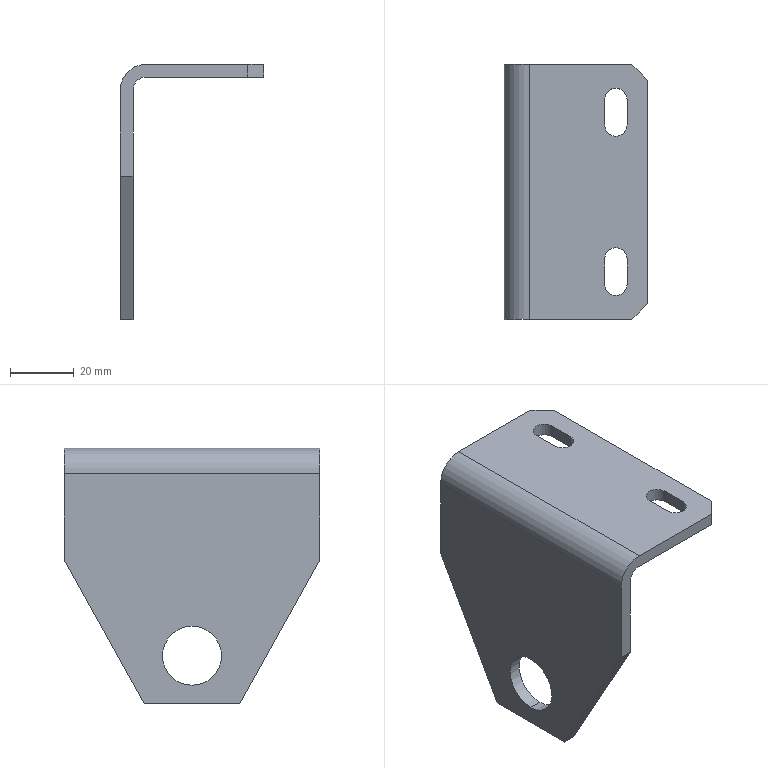Part | SolidWorks | features ICE 3, Chamfer 2, Fillet 2, Extrusion 1, HoleWzd 1 | 1 solid | 24 faces | box 45 x 80 x 80 mm | volume 31465 mm3 | plane 16 | cylinder 8 | commonest cylinder face diameters 7 x4 18.5 x2 8 x1 16 x1
STEP:
#1=CARTESIAN_POINT('',(-4.,40.,24.25));
#2=VERTEX_POINT('',#1);
#3=CARTESIAN_POINT('',(-4.,40.,5.75));
#4=VERTEX_POINT('',#3);
#5=CARTESIAN_POINT('',(-4.,40.,15.));
#6=DIRECTION('',(1.,0.,0.));
#7=DIRECTION('',(0.,0.,-1.));
#8=AXIS2_PLACEMENT_3D('',#5,#6,#7);
#9=CIRCLE('',#8,9.25);
#10=EDGE_CURVE('',#2,#4,#9,.T.);
#11=ORIENTED_EDGE('',*,*,#10,.F.);
#12=CARTESIAN_POINT('',(0.,40.,24.25));
#13=VERTEX_POINT('',#12);
#14=CARTESIAN_POINT('',(0.,40.,24.25));
#15=DIRECTION('',(1.,0.,0.));
#16=VECTOR('',#15,1000.);
#17=LINE('',#14,#16);
#18=EDGE_CURVE('',#2,#13,#17,.T.);
#19=ORIENTED_EDGE('',*,*,#18,.T.);
#20=CARTESIAN_POINT('',(0.,40.,5.75));
#21=VERTEX_POINT('',#20);
#22=CARTESIAN_POINT('',(0.,40.,15.));
#23=DIRECTION('',(1.,0.,0.));
#24=DIRECTION('',(0.,0.,-1.));
#25=AXIS2_PLACEMENT_3D('',#22,#23,#24);
#26=CIRCLE('',#25,9.25);
#27=EDGE_CURVE('',#13,#21,#26,.T.);
#28=ORIENTED_EDGE('',*,*,#27,.T.);
#29=CARTESIAN_POINT('',(0.,40.,5.75));
#30=DIRECTION('',(1.,0.,0.));
#31=VECTOR('',#30,1000.);
#32=LINE('',#29,#31);
#33=EDGE_CURVE('',#4,#21,#32,.T.);
#34=ORIENTED_EDGE('',*,*,#33,.F.);
#35=EDGE_LOOP('',(#11,#19,#28,#34));
#36=FACE_OUTER_BOUND('',#35,.T.);
#37=CARTESIAN_POINT('',(0.,40.,15.));
#38=DIRECTION('',(1.,0.,0.));
#39=DIRECTION('',(0.,0.,-1.));
#40=AXIS2_PLACEMENT_3D('',#37,#38,#39);
#41=CYLINDRICAL_SURFACE('',#40,9.25);
#42=ADVANCED_FACE('',(#36),#41,.F.);
#43=CARTESIAN_POINT('',(-4.,0.,72.));
#44=VERTEX_POINT('',#43);
#45=CARTESIAN_POINT('',(-4.,0.,45.));
#46=VERTEX_POINT('',#45);
#47=CARTESIAN_POINT('',(-4.,0.,80.));
#48=DIRECTION('',(0.,0.,-1.));
#49=VECTOR('',#48,1000.);
#50=LINE('',#47,#49);
#51=EDGE_CURVE('',#44,#46,#50,.T.);
#52=ORIENTED_EDGE('',*,*,#51,.F.);
#53=CARTESIAN_POINT('',(-4.,80.,72.));
#54=VERTEX_POINT('',#53);
#55=CARTESIAN_POINT('',(-4.,0.,72.));
#56=DIRECTION('',(0.,1.,0.));
#57=VECTOR('',#56,1000.);
#58=LINE('',#55,#57);
#59=EDGE_CURVE('',#44,#54,#58,.T.);
#60=ORIENTED_EDGE('',*,*,#59,.T.);
#61=CARTESIAN_POINT('',(-4.,80.,45.));
#62=VERTEX_POINT('',#61);
#63=CARTESIAN_POINT('',(-4.,80.,45.));
#64=DIRECTION('',(0.,0.,1.));
#65=VECTOR('',#64,1000.);
#66=LINE('',#63,#65);
#67=EDGE_CURVE('',#62,#54,#66,.T.);
#68=ORIENTED_EDGE('',*,*,#67,.F.);
#69=CARTESIAN_POINT('',(-4.,55.,0.));
#70=VERTEX_POINT('',#69);
#71=CARTESIAN_POINT('',(-4.,40.,-27.));
#72=DIRECTION('',(0.,0.4856,0.8742));
#73=VECTOR('',#72,1000.);
#74=LINE('',#71,#73);
#75=EDGE_CURVE('',#70,#62,#74,.T.);
#76=ORIENTED_EDGE('',*,*,#75,.F.);
#77=CARTESIAN_POINT('',(-4.,25.,0.));
#78=VERTEX_POINT('',#77);
#79=CARTESIAN_POINT('',(-4.,0.,0.));
#80=DIRECTION('',(0.,-1.,0.));
#81=VECTOR('',#80,1000.);
#82=LINE('',#79,#81);
#83=EDGE_CURVE('',#70,#78,#82,.T.);
#84=ORIENTED_EDGE('',*,*,#83,.T.);
#85=CARTESIAN_POINT('',(-4.,0.,45.));
#86=DIRECTION('',(0.,0.4856,-0.8742));
#87=VECTOR('',#86,1000.);
#88=LINE('',#85,#87);
#89=EDGE_CURVE('',#46,#78,#88,.T.);
#90=ORIENTED_EDGE('',*,*,#89,.F.);
#91=EDGE_LOOP('',(#52,#60,#68,#76,#84,#90));
#92=FACE_OUTER_BOUND('',#91,.T.);
#93=CARTESIAN_POINT('',(-4.,40.,15.));
#94=DIRECTION('',(1.,0.,0.));
#95=DIRECTION('',(0.,0.,-1.));
#96=AXIS2_PLACEMENT_3D('',#93,#94,#95);
#97=CIRCLE('',#96,9.25);
#98=EDGE_CURVE('',#4,#2,#97,.T.);
#99=ORIENTED_EDGE('',*,*,#98,.T.);
#100=ORIENTED_EDGE('',*,*,#10,.T.);
#101=EDGE_LOOP('',(#99,#100));
#102=FACE_BOUND('',#101,.T.);
#103=CARTESIAN_POINT('',(-4.,0.,0.));
#104=DIRECTION('',(-1.,0.,0.));
#105=DIRECTION('',(0.,0.,1.));
#106=AXIS2_PLACEMENT_3D('',#103,#104,#105);
#107=PLANE('',#106);
#108=ADVANCED_FACE('',(#92,#102),#107,.T.);
#109=CARTESIAN_POINT('',(0.,40.,15.));
#110=DIRECTION('',(1.,0.,0.));
#111=DIRECTION('',(0.,0.,-1.));
#112=AXIS2_PLACEMENT_3D('',#109,#110,#111);
#113=CIRCLE('',#112,9.25);
#114=EDGE_CURVE('',#21,#13,#113,.T.);
#115=ORIENTED_EDGE('',*,*,#114,.F.);
#116=ORIENTED_EDGE('',*,*,#27,.F.);
#117=EDGE_LOOP('',(#115,#116));
#118=FACE_BOUND('',#117,.T.);
#119=CARTESIAN_POINT('',(0.,80.,45.));
#120=VERTEX_POINT('',#119);
#121=CARTESIAN_POINT('',(0.,80.,72.));
#122=VERTEX_POINT('',#121);
#123=CARTESIAN_POINT('',(0.,80.,45.));
#124=DIRECTION('',(0.,0.,1.));
#125=VECTOR('',#124,1000.);
#126=LINE('',#123,#125);
#127=EDGE_CURVE('',#120,#122,#126,.T.);
#128=ORIENTED_EDGE('',*,*,#127,.T.);
#129=CARTESIAN_POINT('',(0.,0.,72.));
#130=VERTEX_POINT('',#129);
#131=CARTESIAN_POINT('',(0.,0.,72.));
#132=DIRECTION('',(0.,-1.,0.));
#133=VECTOR('',#132,1000.);
#134=LINE('',#131,#133);
#135=EDGE_CURVE('',#122,#130,#134,.T.);
#136=ORIENTED_EDGE('',*,*,#135,.T.);
#137=CARTESIAN_POINT('',(0.,0.,45.));
#138=VERTEX_POINT('',#137);
#139=CARTESIAN_POINT('',(0.,0.,80.));
#140=DIRECTION('',(0.,0.,-1.));
#141=VECTOR('',#140,1000.);
#142=LINE('',#139,#141);
#143=EDGE_CURVE('',#130,#138,#142,.T.);
#144=ORIENTED_EDGE('',*,*,#143,.T.);
#145=CARTESIAN_POINT('',(0.,25.,0.));
#146=VERTEX_POINT('',#145);
#147=CARTESIAN_POINT('',(0.,0.,45.));
#148=DIRECTION('',(0.,0.4856,-0.8742));
#149=VECTOR('',#148,1000.);
#150=LINE('',#147,#149);
#151=EDGE_CURVE('',#138,#146,#150,.T.);
#152=ORIENTED_EDGE('',*,*,#151,.T.);
#153=CARTESIAN_POINT('',(0.,55.,0.));
#154=VERTEX_POINT('',#153);
#155=CARTESIAN_POINT('',(0.,25.,0.));
#156=DIRECTION('',(0.,1.,0.));
#157=VECTOR('',#156,1000.);
#158=LINE('',#155,#157);
#159=EDGE_CURVE('',#146,#154,#158,.T.);
#160=ORIENTED_EDGE('',*,*,#159,.T.);
#161=CARTESIAN_POINT('',(0.,40.,-27.));
#162=DIRECTION('',(0.,0.4856,0.8742));
#163=VECTOR('',#162,1000.);
#164=LINE('',#161,#163);
#165=EDGE_CURVE('',#154,#120,#164,.T.);
#166=ORIENTED_EDGE('',*,*,#165,.T.);
#167=EDGE_LOOP('',(#128,#136,#144,#152,#160,#166));
#168=FACE_OUTER_BOUND('',#167,.T.);
#169=CARTESIAN_POINT('',(0.,0.,0.));
#170=DIRECTION('',(-1.,0.,0.));
#171=DIRECTION('',(0.,0.,1.));
#172=AXIS2_PLACEMENT_3D('',#169,#170,#171);
#173=PLANE('',#172);
#174=ADVANCED_FACE('',(#118,#168),#173,.F.);
#175=CARTESIAN_POINT('',(4.,0.,80.));
#176=VERTEX_POINT('',#175);
#177=CARTESIAN_POINT('',(36.,0.,80.));
#178=VERTEX_POINT('',#177);
#179=CARTESIAN_POINT('',(-4.,0.,80.));
#180=DIRECTION('',(1.,0.,0.));
#181=VECTOR('',#180,1000.);
#182=LINE('',#179,#181);
#183=EDGE_CURVE('',#176,#178,#182,.T.);
#184=ORIENTED_EDGE('',*,*,#183,.F.);
#185=CARTESIAN_POINT('',(4.,0.,72.));
#186=DIRECTION('',(0.,-1.,0.));
#187=DIRECTION('',(0.,0.,-1.));
#188=AXIS2_PLACEMENT_3D('',#185,#186,#187);
#189=CIRCLE('',#188,8.);
#190=EDGE_CURVE('',#176,#44,#189,.T.);
#191=ORIENTED_EDGE('',*,*,#190,.T.);
#192=ORIENTED_EDGE('',*,*,#51,.T.);
#193=CARTESIAN_POINT('',(-4.,0.,45.));
#194=DIRECTION('',(1.,0.,0.));
#195=VECTOR('',#194,1000.);
#196=LINE('',#193,#195);
#197=EDGE_CURVE('',#46,#138,#196,.T.);
#198=ORIENTED_EDGE('',*,*,#197,.T.);
#199=ORIENTED_EDGE('',*,*,#143,.F.);
#200=CARTESIAN_POINT('',(4.,0.,76.));
#201=VERTEX_POINT('',#200);
#202=CARTESIAN_POINT('',(4.,0.,72.));
#203=DIRECTION('',(0.,1.,0.));
#204=DIRECTION('',(0.,0.,-1.));
#205=AXIS2_PLACEMENT_3D('',#202,#203,#204);
#206=CIRCLE('',#205,4.);
#207=EDGE_CURVE('',#130,#201,#206,.T.);
#208=ORIENTED_EDGE('',*,*,#207,.T.);
#209=CARTESIAN_POINT('',(36.,0.,76.));
#210=VERTEX_POINT('',#209);
#211=CARTESIAN_POINT('',(41.,0.,76.));
#212=DIRECTION('',(-1.,0.,0.));
#213=VECTOR('',#212,1000.);
#214=LINE('',#211,#213);
#215=EDGE_CURVE('',#210,#201,#214,.T.);
#216=ORIENTED_EDGE('',*,*,#215,.F.);
#217=CARTESIAN_POINT('',(36.,0.,80.));
#218=DIRECTION('',(0.,0.,1.));
#219=VECTOR('',#218,1000.);
#220=LINE('',#217,#219);
#221=EDGE_CURVE('',#210,#178,#220,.T.);
#222=ORIENTED_EDGE('',*,*,#221,.T.);
#223=EDGE_LOOP('',(#184,#191,#192,#198,#199,#208,#216,#222));
#224=FACE_OUTER_BOUND('',#223,.T.);
#225=CARTESIAN_POINT('',(-4.,0.,80.));
#226=DIRECTION('',(0.,-1.,0.));
#227=DIRECTION('',(0.,0.,-1.));
#228=AXIS2_PLACEMENT_3D('',#225,#226,#227);
#229=PLANE('',#228);
#230=ADVANCED_FACE('',(#224),#229,.T.);
#231=CARTESIAN_POINT('',(27.5,19.,80.));
#232=VERTEX_POINT('',#231);
#233=CARTESIAN_POINT('',(34.5,19.,80.));
#234=VERTEX_POINT('',#233);
#235=CARTESIAN_POINT('',(31.,19.,80.));
#236=DIRECTION('',(0.,0.,-1.));
#237=DIRECTION('',(-1.,0.,0.));
#238=AXIS2_PLACEMENT_3D('',#235,#236,#237);
#239=CIRCLE('',#238,3.5);
#240=EDGE_CURVE('',#232,#234,#239,.T.);
#241=ORIENTED_EDGE('',*,*,#240,.T.);
#242=CARTESIAN_POINT('',(34.5,11.,80.));
#243=VERTEX_POINT('',#242);
#244=CARTESIAN_POINT('',(34.5,19.,80.));
#245=DIRECTION('',(0.,-1.,0.));
#246=VECTOR('',#245,1000.);
#247=LINE('',#244,#246);
#248=EDGE_CURVE('',#234,#243,#247,.T.);
#249=ORIENTED_EDGE('',*,*,#248,.T.);
#250=CARTESIAN_POINT('',(27.5,11.,80.));
#251=VERTEX_POINT('',#250);
#252=CARTESIAN_POINT('',(31.,11.,80.));
#253=DIRECTION('',(0.,0.,-1.));
#254=DIRECTION('',(-1.,0.,0.));
#255=AXIS2_PLACEMENT_3D('',#252,#253,#254);
#256=CIRCLE('',#255,3.5);
#257=EDGE_CURVE('',#243,#251,#256,.T.);
#258=ORIENTED_EDGE('',*,*,#257,.T.);
#259=CARTESIAN_POINT('',(27.5,11.,80.));
#260=DIRECTION('',(0.,1.,0.));
#261=VECTOR('',#260,1000.);
#262=LINE('',#259,#261);
#263=EDGE_CURVE('',#251,#232,#262,.T.);
#264=ORIENTED_EDGE('',*,*,#263,.T.);
#265=EDGE_LOOP('',(#241,#249,#258,#264));
#266=FACE_BOUND('',#265,.T.);
#267=CARTESIAN_POINT('',(27.5,61.,80.));
#268=VERTEX_POINT('',#267);
#269=CARTESIAN_POINT('',(34.5,61.,80.));
#270=VERTEX_POINT('',#269);
#271=CARTESIAN_POINT('',(31.,61.,80.));
#272=DIRECTION('',(0.,0.,1.));
#273=DIRECTION('',(1.,0.,0.));
#274=AXIS2_PLACEMENT_3D('',#271,#272,#273);
#275=CIRCLE('',#274,3.5);
#276=EDGE_CURVE('',#268,#270,#275,.T.);
#277=ORIENTED_EDGE('',*,*,#276,.F.);
#278=CARTESIAN_POINT('',(27.5,69.,80.));
#279=VERTEX_POINT('',#278);
#280=CARTESIAN_POINT('',(27.5,69.,80.));
#281=DIRECTION('',(0.,-1.,0.));
#282=VECTOR('',#281,1000.);
#283=LINE('',#280,#282);
#284=EDGE_CURVE('',#279,#268,#283,.T.);
#285=ORIENTED_EDGE('',*,*,#284,.F.);
#286=CARTESIAN_POINT('',(34.5,69.,80.));
#287=VERTEX_POINT('',#286);
#288=CARTESIAN_POINT('',(31.,69.,80.));
#289=DIRECTION('',(0.,0.,1.));
#290=DIRECTION('',(1.,0.,0.));
#291=AXIS2_PLACEMENT_3D('',#288,#289,#290);
#292=CIRCLE('',#291,3.5);
#293=EDGE_CURVE('',#287,#279,#292,.T.);
#294=ORIENTED_EDGE('',*,*,#293,.F.);
#295=CARTESIAN_POINT('',(34.5,61.,80.));
#296=DIRECTION('',(0.,1.,0.));
#297=VECTOR('',#296,1000.);
#298=LINE('',#295,#297);
#299=EDGE_CURVE('',#270,#287,#298,.T.);
#300=ORIENTED_EDGE('',*,*,#299,.F.);
#301=EDGE_LOOP('',(#277,#285,#294,#300));
#302=FACE_BOUND('',#301,.T.);
#303=CARTESIAN_POINT('',(4.,80.,80.));
#304=VERTEX_POINT('',#303);
#305=CARTESIAN_POINT('',(36.,80.,80.));
#306=VERTEX_POINT('',#305);
#307=CARTESIAN_POINT('',(-4.,80.,80.));
#308=DIRECTION('',(1.,0.,0.));
#309=VECTOR('',#308,1000.);
#310=LINE('',#307,#309);
#311=EDGE_CURVE('',#304,#306,#310,.T.);
#312=ORIENTED_EDGE('',*,*,#311,.F.);
#313=CARTESIAN_POINT('',(4.,80.,80.));
#314=DIRECTION('',(0.,-1.,0.));
#315=VECTOR('',#314,1000.);
#316=LINE('',#313,#315);
#317=EDGE_CURVE('',#304,#176,#316,.T.);
#318=ORIENTED_EDGE('',*,*,#317,.T.);
#319=ORIENTED_EDGE('',*,*,#183,.T.);
#320=CARTESIAN_POINT('',(41.,5.,80.));
#321=VERTEX_POINT('',#320);
#322=CARTESIAN_POINT('',(56.,20.,80.));
#323=DIRECTION('',(0.7071,0.7071,0.));
#324=VECTOR('',#323,1000.);
#325=LINE('',#322,#324);
#326=EDGE_CURVE('',#178,#321,#325,.T.);
#327=ORIENTED_EDGE('',*,*,#326,.T.);
#328=CARTESIAN_POINT('',(41.,75.,80.));
#329=VERTEX_POINT('',#328);
#330=CARTESIAN_POINT('',(41.,0.,80.));
#331=DIRECTION('',(0.,-1.,0.));
#332=VECTOR('',#331,1000.);
#333=LINE('',#330,#332);
#334=EDGE_CURVE('',#329,#321,#333,.T.);
#335=ORIENTED_EDGE('',*,*,#334,.F.);
#336=CARTESIAN_POINT('',(16.,100.,80.));
#337=DIRECTION('',(-0.7071,0.7071,0.));
#338=VECTOR('',#337,1000.);
#339=LINE('',#336,#338);
#340=EDGE_CURVE('',#329,#306,#339,.T.);
#341=ORIENTED_EDGE('',*,*,#340,.T.);
#342=EDGE_LOOP('',(#312,#318,#319,#327,#335,#341));
#343=FACE_OUTER_BOUND('',#342,.T.);
#344=CARTESIAN_POINT('',(-4.,80.,80.));
#345=DIRECTION('',(0.,0.,1.));
#346=DIRECTION('',(1.,0.,0.));
#347=AXIS2_PLACEMENT_3D('',#344,#345,#346);
#348=PLANE('',#347);
#349=ADVANCED_FACE('',(#266,#302,#343),#348,.T.);
#350=ORIENTED_EDGE('',*,*,#67,.T.);
#351=CARTESIAN_POINT('',(4.,80.,72.));
#352=DIRECTION('',(0.,1.,0.));
#353=DIRECTION('',(0.,0.,1.));
#354=AXIS2_PLACEMENT_3D('',#351,#352,#353);
#355=CIRCLE('',#354,8.);
#356=EDGE_CURVE('',#54,#304,#355,.T.);
#357=ORIENTED_EDGE('',*,*,#356,.T.);
#358=ORIENTED_EDGE('',*,*,#311,.T.);
#359=CARTESIAN_POINT('',(36.,80.,76.));
#360=VERTEX_POINT('',#359);
#361=CARTESIAN_POINT('',(36.,80.,76.));
#362=DIRECTION('',(0.,0.,-1.));
#363=VECTOR('',#362,1000.);
#364=LINE('',#361,#363);
#365=EDGE_CURVE('',#306,#360,#364,.T.);
#366=ORIENTED_EDGE('',*,*,#365,.T.);
#367=CARTESIAN_POINT('',(4.,80.,76.));
#368=VERTEX_POINT('',#367);
#369=CARTESIAN_POINT('',(41.,80.,76.));
#370=DIRECTION('',(-1.,0.,0.));
#371=VECTOR('',#370,1000.);
#372=LINE('',#369,#371);
#373=EDGE_CURVE('',#360,#368,#372,.T.);
#374=ORIENTED_EDGE('',*,*,#373,.T.);
#375=CARTESIAN_POINT('',(4.,80.,72.));
#376=DIRECTION('',(0.,-1.,0.));
#377=DIRECTION('',(0.,0.,1.));
#378=AXIS2_PLACEMENT_3D('',#375,#376,#377);
#379=CIRCLE('',#378,4.);
#380=EDGE_CURVE('',#368,#122,#379,.T.);
#381=ORIENTED_EDGE('',*,*,#380,.T.);
#382=ORIENTED_EDGE('',*,*,#127,.F.);
#383=CARTESIAN_POINT('',(-4.,80.,45.));
#384=DIRECTION('',(1.,0.,0.));
#385=VECTOR('',#384,1000.);
#386=LINE('',#383,#385);
#387=EDGE_CURVE('',#62,#120,#386,.T.);
#388=ORIENTED_EDGE('',*,*,#387,.F.);
#389=EDGE_LOOP('',(#350,#357,#358,#366,#374,#381,#382,#388));
#390=FACE_OUTER_BOUND('',#389,.T.);
#391=CARTESIAN_POINT('',(-4.,80.,45.));
#392=DIRECTION('',(0.,1.,0.));
#393=DIRECTION('',(0.,0.,1.));
#394=AXIS2_PLACEMENT_3D('',#391,#392,#393);
#395=PLANE('',#394);
#396=ADVANCED_FACE('',(#390),#395,.T.);
#397=ORIENTED_EDGE('',*,*,#165,.F.);
#398=CARTESIAN_POINT('',(-4.,55.,0.));
#399=DIRECTION('',(-1.,0.,0.));
#400=VECTOR('',#399,1000.);
#401=LINE('',#398,#400);
#402=EDGE_CURVE('',#154,#70,#401,.T.);
#403=ORIENTED_EDGE('',*,*,#402,.T.);
#404=ORIENTED_EDGE('',*,*,#75,.T.);
#405=ORIENTED_EDGE('',*,*,#387,.T.);
#406=EDGE_LOOP('',(#397,#403,#404,#405));
#407=FACE_OUTER_BOUND('',#406,.T.);
#408=CARTESIAN_POINT('',(-4.,40.,-27.));
#409=DIRECTION('',(0.,0.8742,-0.4856));
#410=DIRECTION('',(0.,0.4856,0.8742));
#411=AXIS2_PLACEMENT_3D('',#408,#409,#410);
#412=PLANE('',#411);
#413=ADVANCED_FACE('',(#407),#412,.T.);
#414=ORIENTED_EDGE('',*,*,#89,.T.);
#415=CARTESIAN_POINT('',(-4.,25.,0.));
#416=DIRECTION('',(1.,0.,0.));
#417=VECTOR('',#416,1000.);
#418=LINE('',#415,#417);
#419=EDGE_CURVE('',#78,#146,#418,.T.);
#420=ORIENTED_EDGE('',*,*,#419,.T.);
#421=ORIENTED_EDGE('',*,*,#151,.F.);
#422=ORIENTED_EDGE('',*,*,#197,.F.);
#423=EDGE_LOOP('',(#414,#420,#421,#422));
#424=FACE_OUTER_BOUND('',#423,.T.);
#425=CARTESIAN_POINT('',(-4.,0.,45.));
#426=DIRECTION('',(0.,-0.8742,-0.4856));
#427=DIRECTION('',(0.,0.4856,-0.8742));
#428=AXIS2_PLACEMENT_3D('',#425,#426,#427);
#429=PLANE('',#428);
#430=ADVANCED_FACE('',(#424),#429,.T.);
#431=CARTESIAN_POINT('',(34.5,19.,76.));
#432=VERTEX_POINT('',#431);
#433=CARTESIAN_POINT('',(34.5,11.,76.));
#434=VERTEX_POINT('',#433);
#435=CARTESIAN_POINT('',(34.5,19.,76.));
#436=DIRECTION('',(0.,-1.,0.));
#437=VECTOR('',#436,1000.);
#438=LINE('',#435,#437);
#439=EDGE_CURVE('',#432,#434,#438,.T.);
#440=ORIENTED_EDGE('',*,*,#439,.F.);
#441=CARTESIAN_POINT('',(27.5,19.,76.));
#442=VERTEX_POINT('',#441);
#443=CARTESIAN_POINT('',(31.,19.,76.));
#444=DIRECTION('',(0.,0.,-1.));
#445=DIRECTION('',(-1.,0.,0.));
#446=AXIS2_PLACEMENT_3D('',#443,#444,#445);
#447=CIRCLE('',#446,3.5);
#448=EDGE_CURVE('',#442,#432,#447,.T.);
#449=ORIENTED_EDGE('',*,*,#448,.F.);
#450=CARTESIAN_POINT('',(27.5,11.,76.));
#451=VERTEX_POINT('',#450);
#452=CARTESIAN_POINT('',(27.5,11.,76.));
#453=DIRECTION('',(0.,1.,0.));
#454=VECTOR('',#453,1000.);
#455=LINE('',#452,#454);
#456=EDGE_CURVE('',#451,#442,#455,.T.);
#457=ORIENTED_EDGE('',*,*,#456,.F.);
#458=CARTESIAN_POINT('',(31.,11.,76.));
#459=DIRECTION('',(0.,0.,-1.));
#460=DIRECTION('',(-1.,0.,0.));
#461=AXIS2_PLACEMENT_3D('',#458,#459,#460);
#462=CIRCLE('',#461,3.5);
#463=EDGE_CURVE('',#434,#451,#462,.T.);
#464=ORIENTED_EDGE('',*,*,#463,.F.);
#465=EDGE_LOOP('',(#440,#449,#457,#464));
#466=FACE_BOUND('',#465,.T.);
#467=CARTESIAN_POINT('',(27.5,69.,76.));
#468=VERTEX_POINT('',#467);
#469=CARTESIAN_POINT('',(27.5,61.,76.));
#470=VERTEX_POINT('',#469);
#471=CARTESIAN_POINT('',(27.5,80.,76.));
#472=DIRECTION('',(0.,-1.,0.));
#473=VECTOR('',#472,1000.);
#474=LINE('',#471,#473);
#475=EDGE_CURVE('',#468,#470,#474,.T.);
#476=ORIENTED_EDGE('',*,*,#475,.T.);
#477=CARTESIAN_POINT('',(34.5,61.,76.));
#478=VERTEX_POINT('',#477);
#479=CARTESIAN_POINT('',(31.,61.,76.));
#480=DIRECTION('',(0.,0.,1.));
#481=DIRECTION('',(1.,0.,0.));
#482=AXIS2_PLACEMENT_3D('',#479,#480,#481);
#483=CIRCLE('',#482,3.5);
#484=EDGE_CURVE('',#470,#478,#483,.T.);
#485=ORIENTED_EDGE('',*,*,#484,.T.);
#486=CARTESIAN_POINT('',(34.5,69.,76.));
#487=VERTEX_POINT('',#486);
#488=CARTESIAN_POINT('',(34.5,80.,76.));
#489=DIRECTION('',(0.,1.,0.));
#490=VECTOR('',#489,1000.);
#491=LINE('',#488,#490);
#492=EDGE_CURVE('',#478,#487,#491,.T.);
#493=ORIENTED_EDGE('',*,*,#492,.T.);
#494=CARTESIAN_POINT('',(31.,69.,76.));
#495=DIRECTION('',(0.,0.,1.));
#496=DIRECTION('',(1.,0.,0.));
#497=AXIS2_PLACEMENT_3D('',#494,#495,#496);
#498=CIRCLE('',#497,3.5);
#499=EDGE_CURVE('',#487,#468,#498,.T.);
#500=ORIENTED_EDGE('',*,*,#499,.T.);
#501=EDGE_LOOP('',(#476,#485,#493,#500));
#502=FACE_BOUND('',#501,.T.);
#503=ORIENTED_EDGE('',*,*,#215,.T.);
#504=CARTESIAN_POINT('',(4.,80.,76.));
#505=DIRECTION('',(0.,1.,0.));
#506=VECTOR('',#505,1000.);
#507=LINE('',#504,#506);
#508=EDGE_CURVE('',#201,#368,#507,.T.);
#509=ORIENTED_EDGE('',*,*,#508,.T.);
#510=ORIENTED_EDGE('',*,*,#373,.F.);
#511=CARTESIAN_POINT('',(41.,75.,76.));
#512=VERTEX_POINT('',#511);
#513=CARTESIAN_POINT('',(41.,75.,76.));
#514=DIRECTION('',(0.7071,-0.7071,0.));
#515=VECTOR('',#514,1000.);
#516=LINE('',#513,#515);
#517=EDGE_CURVE('',#360,#512,#516,.T.);
#518=ORIENTED_EDGE('',*,*,#517,.T.);
#519=CARTESIAN_POINT('',(41.,5.,76.));
#520=VERTEX_POINT('',#519);
#521=CARTESIAN_POINT('',(41.,80.,76.));
#522=DIRECTION('',(0.,1.,0.));
#523=VECTOR('',#522,1000.);
#524=LINE('',#521,#523);
#525=EDGE_CURVE('',#520,#512,#524,.T.);
#526=ORIENTED_EDGE('',*,*,#525,.F.);
#527=CARTESIAN_POINT('',(41.,5.,76.));
#528=DIRECTION('',(-0.7071,-0.7071,0.));
#529=VECTOR('',#528,1000.);
#530=LINE('',#527,#529);
#531=EDGE_CURVE('',#520,#210,#530,.T.);
#532=ORIENTED_EDGE('',*,*,#531,.T.);
#533=EDGE_LOOP('',(#503,#509,#510,#518,#526,#532));
#534=FACE_OUTER_BOUND('',#533,.T.);
#535=CARTESIAN_POINT('',(41.,80.,76.));
#536=DIRECTION('',(0.,0.,1.));
#537=DIRECTION('',(1.,0.,0.));
#538=AXIS2_PLACEMENT_3D('',#535,#536,#537);
#539=PLANE('',#538);
#540=ADVANCED_FACE('',(#466,#502,#534),#539,.F.);
#541=ORIENTED_EDGE('',*,*,#334,.T.);
#542=CARTESIAN_POINT('',(41.,5.,76.));
#543=DIRECTION('',(0.,0.,-1.));
#544=VECTOR('',#543,1000.);
#545=LINE('',#542,#544);
#546=EDGE_CURVE('',#321,#520,#545,.T.);
#547=ORIENTED_EDGE('',*,*,#546,.T.);
#548=ORIENTED_EDGE('',*,*,#525,.T.);
#549=CARTESIAN_POINT('',(41.,75.,80.));
#550=DIRECTION('',(0.,0.,1.));
#551=VECTOR('',#550,1000.);
#552=LINE('',#549,#551);
#553=EDGE_CURVE('',#512,#329,#552,.T.);
#554=ORIENTED_EDGE('',*,*,#553,.T.);
#555=EDGE_LOOP('',(#541,#547,#548,#554));
#556=FACE_OUTER_BOUND('',#555,.T.);
#557=CARTESIAN_POINT('',(41.,0.,0.));
#558=DIRECTION('',(-1.,0.,0.));
#559=DIRECTION('',(0.,0.,1.));
#560=AXIS2_PLACEMENT_3D('',#557,#558,#559);
#561=PLANE('',#560);
#562=ADVANCED_FACE('',(#556),#561,.F.);
#563=CARTESIAN_POINT('',(27.5,61.,-27.));
#564=DIRECTION('',(0.,0.,1.));
#565=VECTOR('',#564,1000.);
#566=LINE('',#563,#565);
#567=EDGE_CURVE('',#470,#268,#566,.T.);
#568=ORIENTED_EDGE('',*,*,#567,.T.);
#569=ORIENTED_EDGE('',*,*,#276,.T.);
#570=CARTESIAN_POINT('',(34.5,61.,-27.));
#571=DIRECTION('',(0.,0.,1.));
#572=VECTOR('',#571,1000.);
#573=LINE('',#570,#572);
#574=EDGE_CURVE('',#478,#270,#573,.T.);
#575=ORIENTED_EDGE('',*,*,#574,.F.);
#576=ORIENTED_EDGE('',*,*,#484,.F.);
#577=EDGE_LOOP('',(#568,#569,#575,#576));
#578=FACE_OUTER_BOUND('',#577,.T.);
#579=CARTESIAN_POINT('',(31.,61.,-27.));
#580=DIRECTION('',(0.,0.,1.));
#581=DIRECTION('',(1.,0.,0.));
#582=AXIS2_PLACEMENT_3D('',#579,#580,#581);
#583=CYLINDRICAL_SURFACE('',#582,3.5);
#584=ADVANCED_FACE('',(#578),#583,.F.);
#585=CARTESIAN_POINT('',(27.5,69.,-27.));
#586=DIRECTION('',(0.,0.,1.));
#587=VECTOR('',#586,1000.);
#588=LINE('',#585,#587);
#589=EDGE_CURVE('',#468,#279,#588,.T.);
#590=ORIENTED_EDGE('',*,*,#589,.T.);
#591=ORIENTED_EDGE('',*,*,#284,.T.);
#592=ORIENTED_EDGE('',*,*,#567,.F.);
#593=ORIENTED_EDGE('',*,*,#475,.F.);
#594=EDGE_LOOP('',(#590,#591,#592,#593));
#595=FACE_OUTER_BOUND('',#594,.T.);
#596=CARTESIAN_POINT('',(27.5,69.,-27.));
#597=DIRECTION('',(-1.,0.,0.));
#598=DIRECTION('',(0.,-1.,0.));
#599=AXIS2_PLACEMENT_3D('',#596,#597,#598);
#600=PLANE('',#599);
#601=ADVANCED_FACE('',(#595),#600,.F.);
#602=CARTESIAN_POINT('',(34.5,69.,-27.));
#603=DIRECTION('',(0.,0.,1.));
#604=VECTOR('',#603,1000.);
#605=LINE('',#602,#604);
#606=EDGE_CURVE('',#487,#287,#605,.T.);
#607=ORIENTED_EDGE('',*,*,#606,.T.);
#608=ORIENTED_EDGE('',*,*,#293,.T.);
#609=ORIENTED_EDGE('',*,*,#589,.F.);
#610=ORIENTED_EDGE('',*,*,#499,.F.);
#611=EDGE_LOOP('',(#607,#608,#609,#610));
#612=FACE_OUTER_BOUND('',#611,.T.);
#613=CARTESIAN_POINT('',(31.,69.,-27.));
#614=DIRECTION('',(0.,0.,1.));
#615=DIRECTION('',(1.,0.,0.));
#616=AXIS2_PLACEMENT_3D('',#613,#614,#615);
#617=CYLINDRICAL_SURFACE('',#616,3.5);
#618=ADVANCED_FACE('',(#612),#617,.F.);
#619=ORIENTED_EDGE('',*,*,#574,.T.);
#620=ORIENTED_EDGE('',*,*,#299,.T.);
#621=ORIENTED_EDGE('',*,*,#606,.F.);
#622=ORIENTED_EDGE('',*,*,#492,.F.);
#623=EDGE_LOOP('',(#619,#620,#621,#622));
#624=FACE_OUTER_BOUND('',#623,.T.);
#625=CARTESIAN_POINT('',(34.5,61.,-27.));
#626=DIRECTION('',(1.,0.,0.));
#627=DIRECTION('',(0.,0.,-1.));
#628=AXIS2_PLACEMENT_3D('',#625,#626,#627);
#629=PLANE('',#628);
#630=ADVANCED_FACE('',(#624),#629,.F.);
#631=ORIENTED_EDGE('',*,*,#448,.T.);
#632=CARTESIAN_POINT('',(34.5,19.,80.));
#633=DIRECTION('',(0.,0.,-1.));
#634=VECTOR('',#633,1000.);
#635=LINE('',#632,#634);
#636=EDGE_CURVE('',#234,#432,#635,.T.);
#637=ORIENTED_EDGE('',*,*,#636,.F.);
#638=ORIENTED_EDGE('',*,*,#240,.F.);
#639=CARTESIAN_POINT('',(27.5,19.,80.));
#640=DIRECTION('',(0.,0.,-1.));
#641=VECTOR('',#640,1000.);
#642=LINE('',#639,#641);
#643=EDGE_CURVE('',#232,#442,#642,.T.);
#644=ORIENTED_EDGE('',*,*,#643,.T.);
#645=EDGE_LOOP('',(#631,#637,#638,#644));
#646=FACE_OUTER_BOUND('',#645,.T.);
#647=CARTESIAN_POINT('',(31.,19.,80.));
#648=DIRECTION('',(0.,0.,-1.));
#649=DIRECTION('',(-1.,0.,0.));
#650=AXIS2_PLACEMENT_3D('',#647,#648,#649);
#651=CYLINDRICAL_SURFACE('',#650,3.5);
#652=ADVANCED_FACE('',(#646),#651,.F.);
#653=ORIENTED_EDGE('',*,*,#456,.T.);
#654=ORIENTED_EDGE('',*,*,#643,.F.);
#655=ORIENTED_EDGE('',*,*,#263,.F.);
#656=CARTESIAN_POINT('',(27.5,11.,80.));
#657=DIRECTION('',(0.,0.,-1.));
#658=VECTOR('',#657,1000.);
#659=LINE('',#656,#658);
#660=EDGE_CURVE('',#251,#451,#659,.T.);
#661=ORIENTED_EDGE('',*,*,#660,.T.);
#662=EDGE_LOOP('',(#653,#654,#655,#661));
#663=FACE_OUTER_BOUND('',#662,.T.);
#664=CARTESIAN_POINT('',(27.5,11.,80.));
#665=DIRECTION('',(-1.,0.,0.));
#666=DIRECTION('',(0.,-1.,0.));
#667=AXIS2_PLACEMENT_3D('',#664,#665,#666);
#668=PLANE('',#667);
#669=ADVANCED_FACE('',(#663),#668,.F.);
#670=ORIENTED_EDGE('',*,*,#463,.T.);
#671=ORIENTED_EDGE('',*,*,#660,.F.);
#672=ORIENTED_EDGE('',*,*,#257,.F.);
#673=CARTESIAN_POINT('',(34.5,11.,80.));
#674=DIRECTION('',(0.,0.,-1.));
#675=VECTOR('',#674,1000.);
#676=LINE('',#673,#675);
#677=EDGE_CURVE('',#243,#434,#676,.T.);
#678=ORIENTED_EDGE('',*,*,#677,.T.);
#679=EDGE_LOOP('',(#670,#671,#672,#678));
#680=FACE_OUTER_BOUND('',#679,.T.);
#681=CARTESIAN_POINT('',(31.,11.,80.));
#682=DIRECTION('',(0.,0.,-1.));
#683=DIRECTION('',(-1.,0.,0.));
#684=AXIS2_PLACEMENT_3D('',#681,#682,#683);
#685=CYLINDRICAL_SURFACE('',#684,3.5);
#686=ADVANCED_FACE('',(#680),#685,.F.);
#687=ORIENTED_EDGE('',*,*,#439,.T.);
#688=ORIENTED_EDGE('',*,*,#677,.F.);
#689=ORIENTED_EDGE('',*,*,#248,.F.);
#690=ORIENTED_EDGE('',*,*,#636,.T.);
#691=EDGE_LOOP('',(#687,#688,#689,#690));
#692=FACE_OUTER_BOUND('',#691,.T.);
#693=CARTESIAN_POINT('',(34.5,19.,80.));
#694=DIRECTION('',(1.,0.,0.));
#695=DIRECTION('',(0.,1.,0.));
#696=AXIS2_PLACEMENT_3D('',#693,#694,#695);
#697=PLANE('',#696);
#698=ADVANCED_FACE('',(#692),#697,.F.);
#699=ORIENTED_EDGE('',*,*,#18,.F.);
#700=ORIENTED_EDGE('',*,*,#98,.F.);
#701=ORIENTED_EDGE('',*,*,#33,.T.);
#702=ORIENTED_EDGE('',*,*,#114,.T.);
#703=EDGE_LOOP('',(#699,#700,#701,#702));
#704=FACE_OUTER_BOUND('',#703,.T.);
#705=CARTESIAN_POINT('',(0.,40.,15.));
#706=DIRECTION('',(1.,0.,0.));
#707=DIRECTION('',(0.,0.,-1.));
#708=AXIS2_PLACEMENT_3D('',#705,#706,#707);
#709=CYLINDRICAL_SURFACE('',#708,9.25);
#710=ADVANCED_FACE('',(#704),#709,.F.);
#711=ORIENTED_EDGE('',*,*,#326,.F.);
#712=ORIENTED_EDGE('',*,*,#221,.F.);
#713=ORIENTED_EDGE('',*,*,#531,.F.);
#714=ORIENTED_EDGE('',*,*,#546,.F.);
#715=EDGE_LOOP('',(#711,#712,#713,#714));
#716=FACE_OUTER_BOUND('',#715,.T.);
#717=CARTESIAN_POINT('',(41.,5.,0.));
#718=DIRECTION('',(0.7071,-0.7071,0.));
#719=DIRECTION('',(0.,0.,1.));
#720=AXIS2_PLACEMENT_3D('',#717,#718,#719);
#721=PLANE('',#720);
#722=ADVANCED_FACE('',(#716),#721,.T.);
#723=ORIENTED_EDGE('',*,*,#517,.F.);
#724=ORIENTED_EDGE('',*,*,#365,.F.);
#725=ORIENTED_EDGE('',*,*,#340,.F.);
#726=ORIENTED_EDGE('',*,*,#553,.F.);
#727=EDGE_LOOP('',(#723,#724,#725,#726));
#728=FACE_OUTER_BOUND('',#727,.T.);
#729=CARTESIAN_POINT('',(41.,75.,0.));
#730=DIRECTION('',(0.7071,0.7071,0.));
#731=DIRECTION('',(0.,0.,-1.));
#732=AXIS2_PLACEMENT_3D('',#729,#730,#731);
#733=PLANE('',#732);
#734=ADVANCED_FACE('',(#728),#733,.T.);
#735=ORIENTED_EDGE('',*,*,#83,.F.);
#736=ORIENTED_EDGE('',*,*,#402,.F.);
#737=ORIENTED_EDGE('',*,*,#159,.F.);
#738=ORIENTED_EDGE('',*,*,#419,.F.);
#739=EDGE_LOOP('',(#735,#736,#737,#738));
#740=FACE_OUTER_BOUND('',#739,.T.);
#741=CARTESIAN_POINT('',(-4.,25.,0.));
#742=DIRECTION('',(0.,0.,1.));
#743=DIRECTION('',(1.,0.,0.));
#744=AXIS2_PLACEMENT_3D('',#741,#742,#743);
#745=PLANE('',#744);
#746=ADVANCED_FACE('',(#740),#745,.F.);
#747=ORIENTED_EDGE('',*,*,#207,.F.);
#748=ORIENTED_EDGE('',*,*,#135,.F.);
#749=ORIENTED_EDGE('',*,*,#380,.F.);
#750=ORIENTED_EDGE('',*,*,#508,.F.);
#751=EDGE_LOOP('',(#747,#748,#749,#750));
#752=FACE_OUTER_BOUND('',#751,.T.);
#753=CARTESIAN_POINT('',(4.,80.,72.));
#754=DIRECTION('',(0.,-1.,0.));
#755=DIRECTION('',(0.,0.,-1.));
#756=AXIS2_PLACEMENT_3D('',#753,#754,#755);
#757=CYLINDRICAL_SURFACE('',#756,4.);
#758=ADVANCED_FACE('',(#752),#757,.F.);
#759=ORIENTED_EDGE('',*,*,#356,.F.);
#760=ORIENTED_EDGE('',*,*,#59,.F.);
#761=ORIENTED_EDGE('',*,*,#190,.F.);
#762=ORIENTED_EDGE('',*,*,#317,.F.);
#763=EDGE_LOOP('',(#759,#760,#761,#762));
#764=FACE_OUTER_BOUND('',#763,.T.);
#765=CARTESIAN_POINT('',(4.,80.,72.));
#766=DIRECTION('',(0.,-1.,0.));
#767=DIRECTION('',(0.,0.,-1.));
#768=AXIS2_PLACEMENT_3D('',#765,#766,#767);
#769=CYLINDRICAL_SURFACE('',#768,8.);
#770=ADVANCED_FACE('',(#764),#769,.T.);
#771=CLOSED_SHELL('',(#42,#108,#174,#230,#349,#396,#413,#430,#540,#562,#584,#601,#618,#630,#652,#669,#686,#698,#710,#722,#734,#746,#758,#770));
#772=MANIFOLD_SOLID_BREP('',#771);
#773=CARTESIAN_POINT('',(0.,0.,0.));
#774=DIRECTION('',(0.,0.,1.));
#775=DIRECTION('',(1.,0.,0.));
#776=AXIS2_PLACEMENT_3D('',#773,#774,#775);
#777=(LENGTH_UNIT()NAMED_UNIT(*)SI_UNIT(.MILLI.,.METRE.));
#778=UNCERTAINTY_MEASURE_WITH_UNIT(LENGTH_MEASURE(0.00001),#777,'','');
#779=(NAMED_UNIT(*)PLANE_ANGLE_UNIT()SI_UNIT($,.RADIAN.));
#780=(NAMED_UNIT(*)SI_UNIT($,.STERADIAN.)SOLID_ANGLE_UNIT());
#781=(GEOMETRIC_REPRESENTATION_CONTEXT(3)GLOBAL_UNCERTAINTY_ASSIGNED_CONTEXT((#778))GLOBAL_UNIT_ASSIGNED_CONTEXT((#777,#779,#780))REPRESENTATION_CONTEXT('',''));
#782=ADVANCED_BREP_SHAPE_REPRESENTATION('',(#772,#776),#781);